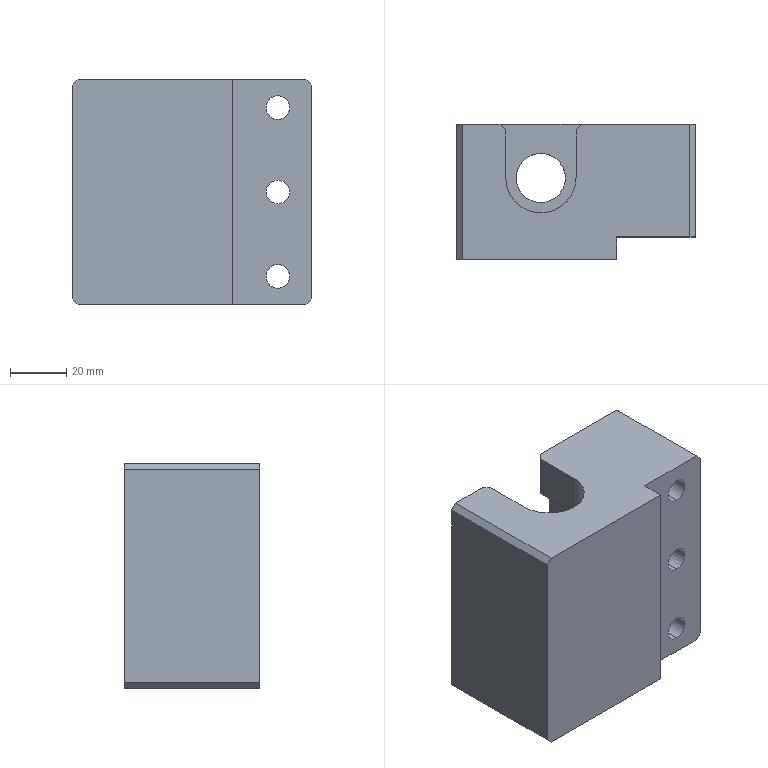Part | SolidWorks | features HoleWzd 2, ICE 2, Chamfer 1, Extrusion 1 | 1 solid | 39 faces | box 85 x 48 x 80 mm | volume 234146 mm3 | plane 23 | cylinder 16 | commonest cylinder face diameters 8.4 x6 15 x6 17.5 x2 25 x1 38 x1
STEP:
#1=CARTESIAN_POINT('',(36.037,-10.191,2.5));
#2=VERTEX_POINT('',#1);
#3=CARTESIAN_POINT('',(36.037,-10.191,17.5));
#4=VERTEX_POINT('',#3);
#5=CARTESIAN_POINT('',(36.037,-10.191,10.));
#6=DIRECTION('',(0.,1.,0.));
#7=DIRECTION('',(0.,0.,1.));
#8=AXIS2_PLACEMENT_3D('',#5,#6,#7);
#9=CIRCLE('',#8,7.5);
#10=EDGE_CURVE('',#2,#4,#9,.T.);
#11=ORIENTED_EDGE('',*,*,#10,.F.);
#12=CARTESIAN_POINT('',(36.037,9.809,2.5));
#13=VERTEX_POINT('',#12);
#14=CARTESIAN_POINT('',(36.037,9.809,2.5));
#15=DIRECTION('',(0.,1.,0.));
#16=VECTOR('',#15,1000.);
#17=LINE('',#14,#16);
#18=EDGE_CURVE('',#2,#13,#17,.T.);
#19=ORIENTED_EDGE('',*,*,#18,.T.);
#20=CARTESIAN_POINT('',(36.037,9.809,17.5));
#21=VERTEX_POINT('',#20);
#22=CARTESIAN_POINT('',(36.037,9.809,10.));
#23=DIRECTION('',(0.,1.,0.));
#24=DIRECTION('',(0.,0.,1.));
#25=AXIS2_PLACEMENT_3D('',#22,#23,#24);
#26=CIRCLE('',#25,7.5);
#27=EDGE_CURVE('',#13,#21,#26,.T.);
#28=ORIENTED_EDGE('',*,*,#27,.T.);
#29=CARTESIAN_POINT('',(36.037,9.809,17.5));
#30=DIRECTION('',(0.,1.,0.));
#31=VECTOR('',#30,1000.);
#32=LINE('',#29,#31);
#33=EDGE_CURVE('',#4,#21,#32,.T.);
#34=ORIENTED_EDGE('',*,*,#33,.F.);
#35=EDGE_LOOP('',(#11,#19,#28,#34));
#36=FACE_OUTER_BOUND('',#35,.T.);
#37=CARTESIAN_POINT('',(36.037,9.809,10.));
#38=DIRECTION('',(0.,1.,0.));
#39=DIRECTION('',(0.,0.,1.));
#40=AXIS2_PLACEMENT_3D('',#37,#38,#39);
#41=CYLINDRICAL_SURFACE('',#40,7.5);
#42=ADVANCED_FACE('',(#36),#41,.F.);
#43=CARTESIAN_POINT('',(36.037,-30.191,5.8));
#44=VERTEX_POINT('',#43);
#45=CARTESIAN_POINT('',(36.037,-30.191,14.2));
#46=VERTEX_POINT('',#45);
#47=CARTESIAN_POINT('',(36.037,-30.191,10.));
#48=DIRECTION('',(0.,1.,0.));
#49=DIRECTION('',(0.,0.,1.));
#50=AXIS2_PLACEMENT_3D('',#47,#48,#49);
#51=CIRCLE('',#50,4.2);
#52=EDGE_CURVE('',#44,#46,#51,.T.);
#53=ORIENTED_EDGE('',*,*,#52,.F.);
#54=CARTESIAN_POINT('',(36.037,-10.191,5.8));
#55=VERTEX_POINT('',#54);
#56=CARTESIAN_POINT('',(36.037,9.809,5.8));
#57=DIRECTION('',(0.,1.,0.));
#58=VECTOR('',#57,1000.);
#59=LINE('',#56,#58);
#60=EDGE_CURVE('',#44,#55,#59,.T.);
#61=ORIENTED_EDGE('',*,*,#60,.T.);
#62=CARTESIAN_POINT('',(36.037,-10.191,14.2));
#63=VERTEX_POINT('',#62);
#64=CARTESIAN_POINT('',(36.037,-10.191,10.));
#65=DIRECTION('',(0.,1.,0.));
#66=DIRECTION('',(0.,0.,1.));
#67=AXIS2_PLACEMENT_3D('',#64,#65,#66);
#68=CIRCLE('',#67,4.2);
#69=EDGE_CURVE('',#55,#63,#68,.T.);
#70=ORIENTED_EDGE('',*,*,#69,.T.);
#71=CARTESIAN_POINT('',(36.037,9.809,14.2));
#72=DIRECTION('',(0.,1.,0.));
#73=VECTOR('',#72,1000.);
#74=LINE('',#71,#73);
#75=EDGE_CURVE('',#46,#63,#74,.T.);
#76=ORIENTED_EDGE('',*,*,#75,.F.);
#77=EDGE_LOOP('',(#53,#61,#70,#76));
#78=FACE_OUTER_BOUND('',#77,.T.);
#79=CARTESIAN_POINT('',(36.037,9.809,10.));
#80=DIRECTION('',(0.,1.,0.));
#81=DIRECTION('',(0.,0.,1.));
#82=AXIS2_PLACEMENT_3D('',#79,#80,#81);
#83=CYLINDRICAL_SURFACE('',#82,4.2);
#84=ADVANCED_FACE('',(#78),#83,.F.);
#85=CARTESIAN_POINT('',(36.037,-10.191,32.5));
#86=VERTEX_POINT('',#85);
#87=CARTESIAN_POINT('',(36.037,-10.191,47.5));
#88=VERTEX_POINT('',#87);
#89=CARTESIAN_POINT('',(36.037,-10.191,40.));
#90=DIRECTION('',(0.,1.,0.));
#91=DIRECTION('',(0.,0.,1.));
#92=AXIS2_PLACEMENT_3D('',#89,#90,#91);
#93=CIRCLE('',#92,7.5);
#94=EDGE_CURVE('',#86,#88,#93,.T.);
#95=ORIENTED_EDGE('',*,*,#94,.F.);
#96=CARTESIAN_POINT('',(36.037,9.809,32.5));
#97=VERTEX_POINT('',#96);
#98=CARTESIAN_POINT('',(36.037,9.809,32.5));
#99=DIRECTION('',(0.,1.,0.));
#100=VECTOR('',#99,1000.);
#101=LINE('',#98,#100);
#102=EDGE_CURVE('',#86,#97,#101,.T.);
#103=ORIENTED_EDGE('',*,*,#102,.T.);
#104=CARTESIAN_POINT('',(36.037,9.809,47.5));
#105=VERTEX_POINT('',#104);
#106=CARTESIAN_POINT('',(36.037,9.809,40.));
#107=DIRECTION('',(0.,1.,0.));
#108=DIRECTION('',(0.,0.,1.));
#109=AXIS2_PLACEMENT_3D('',#106,#107,#108);
#110=CIRCLE('',#109,7.5);
#111=EDGE_CURVE('',#97,#105,#110,.T.);
#112=ORIENTED_EDGE('',*,*,#111,.T.);
#113=CARTESIAN_POINT('',(36.037,9.809,47.5));
#114=DIRECTION('',(0.,1.,0.));
#115=VECTOR('',#114,1000.);
#116=LINE('',#113,#115);
#117=EDGE_CURVE('',#88,#105,#116,.T.);
#118=ORIENTED_EDGE('',*,*,#117,.F.);
#119=EDGE_LOOP('',(#95,#103,#112,#118));
#120=FACE_OUTER_BOUND('',#119,.T.);
#121=CARTESIAN_POINT('',(36.037,9.809,40.));
#122=DIRECTION('',(0.,1.,0.));
#123=DIRECTION('',(0.,0.,1.));
#124=AXIS2_PLACEMENT_3D('',#121,#122,#123);
#125=CYLINDRICAL_SURFACE('',#124,7.5);
#126=ADVANCED_FACE('',(#120),#125,.F.);
#127=CARTESIAN_POINT('',(36.037,-30.191,35.8));
#128=VERTEX_POINT('',#127);
#129=CARTESIAN_POINT('',(36.037,-30.191,44.2));
#130=VERTEX_POINT('',#129);
#131=CARTESIAN_POINT('',(36.037,-30.191,40.));
#132=DIRECTION('',(0.,1.,0.));
#133=DIRECTION('',(0.,0.,1.));
#134=AXIS2_PLACEMENT_3D('',#131,#132,#133);
#135=CIRCLE('',#134,4.2);
#136=EDGE_CURVE('',#128,#130,#135,.T.);
#137=ORIENTED_EDGE('',*,*,#136,.F.);
#138=CARTESIAN_POINT('',(36.037,-10.191,35.8));
#139=VERTEX_POINT('',#138);
#140=CARTESIAN_POINT('',(36.037,9.809,35.8));
#141=DIRECTION('',(0.,1.,0.));
#142=VECTOR('',#141,1000.);
#143=LINE('',#140,#142);
#144=EDGE_CURVE('',#128,#139,#143,.T.);
#145=ORIENTED_EDGE('',*,*,#144,.T.);
#146=CARTESIAN_POINT('',(36.037,-10.191,44.2));
#147=VERTEX_POINT('',#146);
#148=CARTESIAN_POINT('',(36.037,-10.191,40.));
#149=DIRECTION('',(0.,1.,0.));
#150=DIRECTION('',(0.,0.,1.));
#151=AXIS2_PLACEMENT_3D('',#148,#149,#150);
#152=CIRCLE('',#151,4.2);
#153=EDGE_CURVE('',#139,#147,#152,.T.);
#154=ORIENTED_EDGE('',*,*,#153,.T.);
#155=CARTESIAN_POINT('',(36.037,9.809,44.2));
#156=DIRECTION('',(0.,1.,0.));
#157=VECTOR('',#156,1000.);
#158=LINE('',#155,#157);
#159=EDGE_CURVE('',#130,#147,#158,.T.);
#160=ORIENTED_EDGE('',*,*,#159,.F.);
#161=EDGE_LOOP('',(#137,#145,#154,#160));
#162=FACE_OUTER_BOUND('',#161,.T.);
#163=CARTESIAN_POINT('',(36.037,9.809,40.));
#164=DIRECTION('',(0.,1.,0.));
#165=DIRECTION('',(0.,0.,1.));
#166=AXIS2_PLACEMENT_3D('',#163,#164,#165);
#167=CYLINDRICAL_SURFACE('',#166,4.2);
#168=ADVANCED_FACE('',(#162),#167,.F.);
#169=CARTESIAN_POINT('',(36.037,-10.191,62.5));
#170=VERTEX_POINT('',#169);
#171=CARTESIAN_POINT('',(36.037,-10.191,77.5));
#172=VERTEX_POINT('',#171);
#173=CARTESIAN_POINT('',(36.037,-10.191,70.));
#174=DIRECTION('',(0.,1.,0.));
#175=DIRECTION('',(0.,0.,1.));
#176=AXIS2_PLACEMENT_3D('',#173,#174,#175);
#177=CIRCLE('',#176,7.5);
#178=EDGE_CURVE('',#170,#172,#177,.T.);
#179=ORIENTED_EDGE('',*,*,#178,.F.);
#180=CARTESIAN_POINT('',(36.037,9.809,62.5));
#181=VERTEX_POINT('',#180);
#182=CARTESIAN_POINT('',(36.037,9.809,62.5));
#183=DIRECTION('',(0.,1.,0.));
#184=VECTOR('',#183,1000.);
#185=LINE('',#182,#184);
#186=EDGE_CURVE('',#170,#181,#185,.T.);
#187=ORIENTED_EDGE('',*,*,#186,.T.);
#188=CARTESIAN_POINT('',(36.037,9.809,77.5));
#189=VERTEX_POINT('',#188);
#190=CARTESIAN_POINT('',(36.037,9.809,70.));
#191=DIRECTION('',(0.,1.,0.));
#192=DIRECTION('',(0.,0.,1.));
#193=AXIS2_PLACEMENT_3D('',#190,#191,#192);
#194=CIRCLE('',#193,7.5);
#195=EDGE_CURVE('',#181,#189,#194,.T.);
#196=ORIENTED_EDGE('',*,*,#195,.T.);
#197=CARTESIAN_POINT('',(36.037,9.809,77.5));
#198=DIRECTION('',(0.,1.,0.));
#199=VECTOR('',#198,1000.);
#200=LINE('',#197,#199);
#201=EDGE_CURVE('',#172,#189,#200,.T.);
#202=ORIENTED_EDGE('',*,*,#201,.F.);
#203=EDGE_LOOP('',(#179,#187,#196,#202));
#204=FACE_OUTER_BOUND('',#203,.T.);
#205=CARTESIAN_POINT('',(36.037,9.809,70.));
#206=DIRECTION('',(0.,1.,0.));
#207=DIRECTION('',(0.,0.,1.));
#208=AXIS2_PLACEMENT_3D('',#205,#206,#207);
#209=CYLINDRICAL_SURFACE('',#208,7.5);
#210=ADVANCED_FACE('',(#204),#209,.F.);
#211=CARTESIAN_POINT('',(36.037,-30.191,65.8));
#212=VERTEX_POINT('',#211);
#213=CARTESIAN_POINT('',(36.037,-30.191,74.2));
#214=VERTEX_POINT('',#213);
#215=CARTESIAN_POINT('',(36.037,-30.191,70.));
#216=DIRECTION('',(0.,1.,0.));
#217=DIRECTION('',(0.,0.,1.));
#218=AXIS2_PLACEMENT_3D('',#215,#216,#217);
#219=CIRCLE('',#218,4.2);
#220=EDGE_CURVE('',#212,#214,#219,.T.);
#221=ORIENTED_EDGE('',*,*,#220,.F.);
#222=CARTESIAN_POINT('',(36.037,-10.191,65.8));
#223=VERTEX_POINT('',#222);
#224=CARTESIAN_POINT('',(36.037,9.809,65.8));
#225=DIRECTION('',(0.,1.,0.));
#226=VECTOR('',#225,1000.);
#227=LINE('',#224,#226);
#228=EDGE_CURVE('',#212,#223,#227,.T.);
#229=ORIENTED_EDGE('',*,*,#228,.T.);
#230=CARTESIAN_POINT('',(36.037,-10.191,74.2));
#231=VERTEX_POINT('',#230);
#232=CARTESIAN_POINT('',(36.037,-10.191,70.));
#233=DIRECTION('',(0.,1.,0.));
#234=DIRECTION('',(0.,0.,1.));
#235=AXIS2_PLACEMENT_3D('',#232,#233,#234);
#236=CIRCLE('',#235,4.2);
#237=EDGE_CURVE('',#223,#231,#236,.T.);
#238=ORIENTED_EDGE('',*,*,#237,.T.);
#239=CARTESIAN_POINT('',(36.037,9.809,74.2));
#240=DIRECTION('',(0.,1.,0.));
#241=VECTOR('',#240,1000.);
#242=LINE('',#239,#241);
#243=EDGE_CURVE('',#214,#231,#242,.T.);
#244=ORIENTED_EDGE('',*,*,#243,.F.);
#245=EDGE_LOOP('',(#221,#229,#238,#244));
#246=FACE_OUTER_BOUND('',#245,.T.);
#247=CARTESIAN_POINT('',(36.037,9.809,70.));
#248=DIRECTION('',(0.,1.,0.));
#249=DIRECTION('',(0.,0.,1.));
#250=AXIS2_PLACEMENT_3D('',#247,#248,#249);
#251=CYLINDRICAL_SURFACE('',#250,4.2);
#252=ADVANCED_FACE('',(#246),#251,.F.);
#253=CARTESIAN_POINT('',(-15.713,-9.191,0.));
#254=VERTEX_POINT('',#253);
#255=CARTESIAN_POINT('',(1.787,-9.191,0.));
#256=VERTEX_POINT('',#255);
#257=CARTESIAN_POINT('',(-6.963,-9.191,0.));
#258=DIRECTION('',(0.,0.,1.));
#259=DIRECTION('',(1.,0.,0.));
#260=AXIS2_PLACEMENT_3D('',#257,#258,#259);
#261=CIRCLE('',#260,8.75);
#262=EDGE_CURVE('',#254,#256,#261,.T.);
#263=ORIENTED_EDGE('',*,*,#262,.F.);
#264=CARTESIAN_POINT('',(-15.713,-9.191,33.));
#265=VERTEX_POINT('',#264);
#266=CARTESIAN_POINT('',(-15.713,-9.191,33.));
#267=DIRECTION('',(0.,0.,1.));
#268=VECTOR('',#267,1000.);
#269=LINE('',#266,#268);
#270=EDGE_CURVE('',#254,#265,#269,.T.);
#271=ORIENTED_EDGE('',*,*,#270,.T.);
#272=CARTESIAN_POINT('',(1.787,-9.191,33.));
#273=VERTEX_POINT('',#272);
#274=CARTESIAN_POINT('',(-6.963,-9.191,33.));
#275=DIRECTION('',(0.,0.,1.));
#276=DIRECTION('',(1.,0.,0.));
#277=AXIS2_PLACEMENT_3D('',#274,#275,#276);
#278=CIRCLE('',#277,8.75);
#279=EDGE_CURVE('',#265,#273,#278,.T.);
#280=ORIENTED_EDGE('',*,*,#279,.T.);
#281=CARTESIAN_POINT('',(1.787,-9.191,33.));
#282=DIRECTION('',(0.,0.,1.));
#283=VECTOR('',#282,1000.);
#284=LINE('',#281,#283);
#285=EDGE_CURVE('',#256,#273,#284,.T.);
#286=ORIENTED_EDGE('',*,*,#285,.F.);
#287=EDGE_LOOP('',(#263,#271,#280,#286));
#288=FACE_OUTER_BOUND('',#287,.T.);
#289=CARTESIAN_POINT('',(-6.963,-9.191,33.));
#290=DIRECTION('',(0.,0.,1.));
#291=DIRECTION('',(1.,0.,0.));
#292=AXIS2_PLACEMENT_3D('',#289,#290,#291);
#293=CYLINDRICAL_SURFACE('',#292,8.75);
#294=ADVANCED_FACE('',(#288),#293,.F.);
#295=CARTESIAN_POINT('',(36.037,9.809,10.));
#296=DIRECTION('',(0.,1.,0.));
#297=DIRECTION('',(0.,0.,1.));
#298=AXIS2_PLACEMENT_3D('',#295,#296,#297);
#299=CIRCLE('',#298,7.5);
#300=EDGE_CURVE('',#21,#13,#299,.T.);
#301=ORIENTED_EDGE('',*,*,#300,.F.);
#302=ORIENTED_EDGE('',*,*,#27,.F.);
#303=EDGE_LOOP('',(#301,#302));
#304=FACE_BOUND('',#303,.T.);
#305=CARTESIAN_POINT('',(36.037,9.809,40.));
#306=DIRECTION('',(0.,1.,0.));
#307=DIRECTION('',(0.,0.,1.));
#308=AXIS2_PLACEMENT_3D('',#305,#306,#307);
#309=CIRCLE('',#308,7.5);
#310=EDGE_CURVE('',#105,#97,#309,.T.);
#311=ORIENTED_EDGE('',*,*,#310,.F.);
#312=ORIENTED_EDGE('',*,*,#111,.F.);
#313=EDGE_LOOP('',(#311,#312));
#314=FACE_BOUND('',#313,.T.);
#315=CARTESIAN_POINT('',(36.037,9.809,70.));
#316=DIRECTION('',(0.,1.,0.));
#317=DIRECTION('',(0.,0.,1.));
#318=AXIS2_PLACEMENT_3D('',#315,#316,#317);
#319=CIRCLE('',#318,7.5);
#320=EDGE_CURVE('',#189,#181,#319,.T.);
#321=ORIENTED_EDGE('',*,*,#320,.F.);
#322=ORIENTED_EDGE('',*,*,#195,.F.);
#323=EDGE_LOOP('',(#321,#322));
#324=FACE_BOUND('',#323,.T.);
#325=CARTESIAN_POINT('',(48.037,9.809,78.));
#326=VERTEX_POINT('',#325);
#327=CARTESIAN_POINT('',(48.037,9.809,2.));
#328=VERTEX_POINT('',#327);
#329=CARTESIAN_POINT('',(48.037,9.809,80.));
#330=DIRECTION('',(0.,0.,-1.));
#331=VECTOR('',#330,1000.);
#332=LINE('',#329,#331);
#333=EDGE_CURVE('',#326,#328,#332,.T.);
#334=ORIENTED_EDGE('',*,*,#333,.T.);
#335=CARTESIAN_POINT('',(46.037,9.809,0.));
#336=VERTEX_POINT('',#335);
#337=CARTESIAN_POINT('',(48.037,9.809,2.));
#338=DIRECTION('',(-0.7071,0.,-0.7071));
#339=VECTOR('',#338,1000.);
#340=LINE('',#337,#339);
#341=EDGE_CURVE('',#328,#336,#340,.T.);
#342=ORIENTED_EDGE('',*,*,#341,.T.);
#343=CARTESIAN_POINT('',(-34.963,9.809,0.));
#344=VERTEX_POINT('',#343);
#345=CARTESIAN_POINT('',(48.037,9.809,0.));
#346=DIRECTION('',(-1.,0.,0.));
#347=VECTOR('',#346,1000.);
#348=LINE('',#345,#347);
#349=EDGE_CURVE('',#336,#344,#348,.T.);
#350=ORIENTED_EDGE('',*,*,#349,.T.);
#351=CARTESIAN_POINT('',(-36.963,9.809,2.));
#352=VERTEX_POINT('',#351);
#353=CARTESIAN_POINT('',(-36.963,9.809,2.));
#354=DIRECTION('',(-0.7071,0.,0.7071));
#355=VECTOR('',#354,1000.);
#356=LINE('',#353,#355);
#357=EDGE_CURVE('',#344,#352,#356,.T.);
#358=ORIENTED_EDGE('',*,*,#357,.T.);
#359=CARTESIAN_POINT('',(-36.963,9.809,78.));
#360=VERTEX_POINT('',#359);
#361=CARTESIAN_POINT('',(-36.963,9.809,80.));
#362=DIRECTION('',(0.,0.,-1.));
#363=VECTOR('',#362,1000.);
#364=LINE('',#361,#363);
#365=EDGE_CURVE('',#360,#352,#364,.T.);
#366=ORIENTED_EDGE('',*,*,#365,.F.);
#367=CARTESIAN_POINT('',(-34.963,9.809,80.));
#368=VERTEX_POINT('',#367);
#369=CARTESIAN_POINT('',(-34.963,9.809,80.));
#370=DIRECTION('',(0.7071,0.,0.7071));
#371=VECTOR('',#370,1000.);
#372=LINE('',#369,#371);
#373=EDGE_CURVE('',#360,#368,#372,.T.);
#374=ORIENTED_EDGE('',*,*,#373,.T.);
#375=CARTESIAN_POINT('',(-21.463,9.809,80.));
#376=VERTEX_POINT('',#375);
#377=CARTESIAN_POINT('',(48.037,9.809,80.));
#378=DIRECTION('',(-1.,0.,0.));
#379=VECTOR('',#378,1000.);
#380=LINE('',#377,#379);
#381=EDGE_CURVE('',#376,#368,#380,.T.);
#382=ORIENTED_EDGE('',*,*,#381,.F.);
#383=CARTESIAN_POINT('',(-21.463,9.809,65.));
#384=VERTEX_POINT('',#383);
#385=CARTESIAN_POINT('',(-21.463,9.809,80.));
#386=DIRECTION('',(0.,0.,-1.));
#387=VECTOR('',#386,1000.);
#388=LINE('',#385,#387);
#389=EDGE_CURVE('',#376,#384,#388,.T.);
#390=ORIENTED_EDGE('',*,*,#389,.T.);
#391=CARTESIAN_POINT('',(-25.963,9.809,65.));
#392=VERTEX_POINT('',#391);
#393=CARTESIAN_POINT('',(-25.963,9.809,65.));
#394=DIRECTION('',(-1.,0.,0.));
#395=VECTOR('',#394,1000.);
#396=LINE('',#393,#395);
#397=EDGE_CURVE('',#384,#392,#396,.T.);
#398=ORIENTED_EDGE('',*,*,#397,.T.);
#399=CARTESIAN_POINT('',(-25.963,9.809,33.));
#400=VERTEX_POINT('',#399);
#401=CARTESIAN_POINT('',(-25.963,9.809,33.));
#402=DIRECTION('',(0.,0.,1.));
#403=VECTOR('',#402,1000.);
#404=LINE('',#401,#403);
#405=EDGE_CURVE('',#400,#392,#404,.T.);
#406=ORIENTED_EDGE('',*,*,#405,.F.);
#407=CARTESIAN_POINT('',(12.037,9.809,33.));
#408=VERTEX_POINT('',#407);
#409=CARTESIAN_POINT('',(-25.963,9.809,33.));
#410=DIRECTION('',(-1.,0.,0.));
#411=VECTOR('',#410,1000.);
#412=LINE('',#409,#411);
#413=EDGE_CURVE('',#408,#400,#412,.T.);
#414=ORIENTED_EDGE('',*,*,#413,.F.);
#415=CARTESIAN_POINT('',(12.037,9.809,65.));
#416=VERTEX_POINT('',#415);
#417=CARTESIAN_POINT('',(12.037,9.809,33.));
#418=DIRECTION('',(0.,0.,1.));
#419=VECTOR('',#418,1000.);
#420=LINE('',#417,#419);
#421=EDGE_CURVE('',#408,#416,#420,.T.);
#422=ORIENTED_EDGE('',*,*,#421,.T.);
#423=CARTESIAN_POINT('',(7.537,9.809,65.));
#424=VERTEX_POINT('',#423);
#425=CARTESIAN_POINT('',(-25.963,9.809,65.));
#426=DIRECTION('',(-1.,0.,0.));
#427=VECTOR('',#426,1000.);
#428=LINE('',#425,#427);
#429=EDGE_CURVE('',#416,#424,#428,.T.);
#430=ORIENTED_EDGE('',*,*,#429,.T.);
#431=CARTESIAN_POINT('',(7.537,9.809,80.));
#432=VERTEX_POINT('',#431);
#433=CARTESIAN_POINT('',(7.537,9.809,80.));
#434=DIRECTION('',(0.,0.,1.));
#435=VECTOR('',#434,1000.);
#436=LINE('',#433,#435);
#437=EDGE_CURVE('',#424,#432,#436,.T.);
#438=ORIENTED_EDGE('',*,*,#437,.T.);
#439=CARTESIAN_POINT('',(46.037,9.809,80.));
#440=VERTEX_POINT('',#439);
#441=CARTESIAN_POINT('',(48.037,9.809,80.));
#442=DIRECTION('',(-1.,0.,0.));
#443=VECTOR('',#442,1000.);
#444=LINE('',#441,#443);
#445=EDGE_CURVE('',#440,#432,#444,.T.);
#446=ORIENTED_EDGE('',*,*,#445,.F.);
#447=CARTESIAN_POINT('',(46.037,9.809,80.));
#448=DIRECTION('',(0.7071,0.,-0.7071));
#449=VECTOR('',#448,1000.);
#450=LINE('',#447,#449);
#451=EDGE_CURVE('',#440,#326,#450,.T.);
#452=ORIENTED_EDGE('',*,*,#451,.T.);
#453=EDGE_LOOP('',(#334,#342,#350,#358,#366,#374,#382,#390,#398,#406,#414,#422,#430,#438,#446,#452));
#454=FACE_OUTER_BOUND('',#453,.T.);
#455=CARTESIAN_POINT('',(48.037,9.809,80.));
#456=DIRECTION('',(0.,-1.,0.));
#457=DIRECTION('',(1.,0.,0.));
#458=AXIS2_PLACEMENT_3D('',#455,#456,#457);
#459=PLANE('',#458);
#460=ADVANCED_FACE('',(#304,#314,#324,#454),#459,.F.);
#461=ORIENTED_EDGE('',*,*,#365,.T.);
#462=CARTESIAN_POINT('',(-36.963,-38.191,2.));
#463=VERTEX_POINT('',#462);
#464=CARTESIAN_POINT('',(-36.963,9.809,2.));
#465=DIRECTION('',(0.,-1.,0.));
#466=VECTOR('',#465,1000.);
#467=LINE('',#464,#466);
#468=EDGE_CURVE('',#352,#463,#467,.T.);
#469=ORIENTED_EDGE('',*,*,#468,.T.);
#470=CARTESIAN_POINT('',(-36.963,-38.191,78.));
#471=VERTEX_POINT('',#470);
#472=CARTESIAN_POINT('',(-36.963,-38.191,80.));
#473=DIRECTION('',(0.,0.,-1.));
#474=VECTOR('',#473,1000.);
#475=LINE('',#472,#474);
#476=EDGE_CURVE('',#471,#463,#475,.T.);
#477=ORIENTED_EDGE('',*,*,#476,.F.);
#478=CARTESIAN_POINT('',(-36.963,9.809,78.));
#479=DIRECTION('',(0.,1.,0.));
#480=VECTOR('',#479,1000.);
#481=LINE('',#478,#480);
#482=EDGE_CURVE('',#471,#360,#481,.T.);
#483=ORIENTED_EDGE('',*,*,#482,.T.);
#484=EDGE_LOOP('',(#461,#469,#477,#483));
#485=FACE_OUTER_BOUND('',#484,.T.);
#486=CARTESIAN_POINT('',(-36.963,9.809,80.));
#487=DIRECTION('',(1.,0.,0.));
#488=DIRECTION('',(0.,0.,-1.));
#489=AXIS2_PLACEMENT_3D('',#486,#487,#488);
#490=PLANE('',#489);
#491=ADVANCED_FACE('',(#485),#490,.F.);
#492=ORIENTED_EDGE('',*,*,#476,.T.);
#493=CARTESIAN_POINT('',(-34.963,-38.191,0.));
#494=VERTEX_POINT('',#493);
#495=CARTESIAN_POINT('',(-36.963,-38.191,2.));
#496=DIRECTION('',(0.7071,0.,-0.7071));
#497=VECTOR('',#496,1000.);
#498=LINE('',#495,#497);
#499=EDGE_CURVE('',#463,#494,#498,.T.);
#500=ORIENTED_EDGE('',*,*,#499,.T.);
#501=CARTESIAN_POINT('',(20.037,-38.191,0.));
#502=VERTEX_POINT('',#501);
#503=CARTESIAN_POINT('',(-36.963,-38.191,0.));
#504=DIRECTION('',(1.,0.,0.));
#505=VECTOR('',#504,1000.);
#506=LINE('',#503,#505);
#507=EDGE_CURVE('',#494,#502,#506,.T.);
#508=ORIENTED_EDGE('',*,*,#507,.T.);
#509=CARTESIAN_POINT('',(20.037,-38.191,80.));
#510=VERTEX_POINT('',#509);
#511=CARTESIAN_POINT('',(20.037,-38.191,80.));
#512=DIRECTION('',(0.,0.,-1.));
#513=VECTOR('',#512,1000.);
#514=LINE('',#511,#513);
#515=EDGE_CURVE('',#510,#502,#514,.T.);
#516=ORIENTED_EDGE('',*,*,#515,.F.);
#517=CARTESIAN_POINT('',(-34.963,-38.191,80.));
#518=VERTEX_POINT('',#517);
#519=CARTESIAN_POINT('',(-36.963,-38.191,80.));
#520=DIRECTION('',(1.,0.,0.));
#521=VECTOR('',#520,1000.);
#522=LINE('',#519,#521);
#523=EDGE_CURVE('',#518,#510,#522,.T.);
#524=ORIENTED_EDGE('',*,*,#523,.F.);
#525=CARTESIAN_POINT('',(-34.963,-38.191,80.));
#526=DIRECTION('',(-0.7071,0.,-0.7071));
#527=VECTOR('',#526,1000.);
#528=LINE('',#525,#527);
#529=EDGE_CURVE('',#518,#471,#528,.T.);
#530=ORIENTED_EDGE('',*,*,#529,.T.);
#531=EDGE_LOOP('',(#492,#500,#508,#516,#524,#530));
#532=FACE_OUTER_BOUND('',#531,.T.);
#533=CARTESIAN_POINT('',(-36.963,-38.191,80.));
#534=DIRECTION('',(0.,1.,0.));
#535=DIRECTION('',(0.,0.,1.));
#536=AXIS2_PLACEMENT_3D('',#533,#534,#535);
#537=PLANE('',#536);
#538=ADVANCED_FACE('',(#532),#537,.F.);
#539=CARTESIAN_POINT('',(20.037,-30.191,0.));
#540=VERTEX_POINT('',#539);
#541=CARTESIAN_POINT('',(20.037,-38.191,0.));
#542=DIRECTION('',(0.,1.,0.));
#543=VECTOR('',#542,1000.);
#544=LINE('',#541,#543);
#545=EDGE_CURVE('',#502,#540,#544,.T.);
#546=ORIENTED_EDGE('',*,*,#545,.T.);
#547=CARTESIAN_POINT('',(20.037,-30.191,80.));
#548=VERTEX_POINT('',#547);
#549=CARTESIAN_POINT('',(20.037,-30.191,80.));
#550=DIRECTION('',(0.,0.,-1.));
#551=VECTOR('',#550,1000.);
#552=LINE('',#549,#551);
#553=EDGE_CURVE('',#548,#540,#552,.T.);
#554=ORIENTED_EDGE('',*,*,#553,.F.);
#555=CARTESIAN_POINT('',(20.037,-38.191,80.));
#556=DIRECTION('',(0.,1.,0.));
#557=VECTOR('',#556,1000.);
#558=LINE('',#555,#557);
#559=EDGE_CURVE('',#510,#548,#558,.T.);
#560=ORIENTED_EDGE('',*,*,#559,.F.);
#561=ORIENTED_EDGE('',*,*,#515,.T.);
#562=EDGE_LOOP('',(#546,#554,#560,#561));
#563=FACE_OUTER_BOUND('',#562,.T.);
#564=CARTESIAN_POINT('',(20.037,-38.191,80.));
#565=DIRECTION('',(-1.,0.,0.));
#566=DIRECTION('',(0.,0.,1.));
#567=AXIS2_PLACEMENT_3D('',#564,#565,#566);
#568=PLANE('',#567);
#569=ADVANCED_FACE('',(#563),#568,.F.);
#570=CARTESIAN_POINT('',(36.037,-30.191,10.));
#571=DIRECTION('',(0.,1.,0.));
#572=DIRECTION('',(0.,0.,1.));
#573=AXIS2_PLACEMENT_3D('',#570,#571,#572);
#574=CIRCLE('',#573,4.2);
#575=EDGE_CURVE('',#46,#44,#574,.T.);
#576=ORIENTED_EDGE('',*,*,#575,.T.);
#577=ORIENTED_EDGE('',*,*,#52,.T.);
#578=EDGE_LOOP('',(#576,#577));
#579=FACE_BOUND('',#578,.T.);
#580=CARTESIAN_POINT('',(36.037,-30.191,40.));
#581=DIRECTION('',(0.,1.,0.));
#582=DIRECTION('',(0.,0.,1.));
#583=AXIS2_PLACEMENT_3D('',#580,#581,#582);
#584=CIRCLE('',#583,4.2);
#585=EDGE_CURVE('',#130,#128,#584,.T.);
#586=ORIENTED_EDGE('',*,*,#585,.T.);
#587=ORIENTED_EDGE('',*,*,#136,.T.);
#588=EDGE_LOOP('',(#586,#587));
#589=FACE_BOUND('',#588,.T.);
#590=CARTESIAN_POINT('',(36.037,-30.191,70.));
#591=DIRECTION('',(0.,1.,0.));
#592=DIRECTION('',(0.,0.,1.));
#593=AXIS2_PLACEMENT_3D('',#590,#591,#592);
#594=CIRCLE('',#593,4.2);
#595=EDGE_CURVE('',#214,#212,#594,.T.);
#596=ORIENTED_EDGE('',*,*,#595,.T.);
#597=ORIENTED_EDGE('',*,*,#220,.T.);
#598=EDGE_LOOP('',(#596,#597));
#599=FACE_BOUND('',#598,.T.);
#600=CARTESIAN_POINT('',(46.037,-30.191,0.));
#601=VERTEX_POINT('',#600);
#602=CARTESIAN_POINT('',(20.037,-30.191,0.));
#603=DIRECTION('',(1.,0.,0.));
#604=VECTOR('',#603,1000.);
#605=LINE('',#602,#604);
#606=EDGE_CURVE('',#540,#601,#605,.T.);
#607=ORIENTED_EDGE('',*,*,#606,.T.);
#608=CARTESIAN_POINT('',(48.037,-30.191,2.));
#609=VERTEX_POINT('',#608);
#610=CARTESIAN_POINT('',(48.037,-30.191,2.));
#611=DIRECTION('',(0.7071,0.,0.7071));
#612=VECTOR('',#611,1000.);
#613=LINE('',#610,#612);
#614=EDGE_CURVE('',#601,#609,#613,.T.);
#615=ORIENTED_EDGE('',*,*,#614,.T.);
#616=CARTESIAN_POINT('',(48.037,-30.191,78.));
#617=VERTEX_POINT('',#616);
#618=CARTESIAN_POINT('',(48.037,-30.191,80.));
#619=DIRECTION('',(0.,0.,-1.));
#620=VECTOR('',#619,1000.);
#621=LINE('',#618,#620);
#622=EDGE_CURVE('',#617,#609,#621,.T.);
#623=ORIENTED_EDGE('',*,*,#622,.F.);
#624=CARTESIAN_POINT('',(46.037,-30.191,80.));
#625=VERTEX_POINT('',#624);
#626=CARTESIAN_POINT('',(46.037,-30.191,80.));
#627=DIRECTION('',(-0.7071,0.,0.7071));
#628=VECTOR('',#627,1000.);
#629=LINE('',#626,#628);
#630=EDGE_CURVE('',#617,#625,#629,.T.);
#631=ORIENTED_EDGE('',*,*,#630,.T.);
#632=CARTESIAN_POINT('',(20.037,-30.191,80.));
#633=DIRECTION('',(1.,0.,0.));
#634=VECTOR('',#633,1000.);
#635=LINE('',#632,#634);
#636=EDGE_CURVE('',#548,#625,#635,.T.);
#637=ORIENTED_EDGE('',*,*,#636,.F.);
#638=ORIENTED_EDGE('',*,*,#553,.T.);
#639=EDGE_LOOP('',(#607,#615,#623,#631,#637,#638));
#640=FACE_OUTER_BOUND('',#639,.T.);
#641=CARTESIAN_POINT('',(20.037,-30.191,80.));
#642=DIRECTION('',(0.,1.,0.));
#643=DIRECTION('',(0.,0.,1.));
#644=AXIS2_PLACEMENT_3D('',#641,#642,#643);
#645=PLANE('',#644);
#646=ADVANCED_FACE('',(#579,#589,#599,#640),#645,.F.);
#647=ORIENTED_EDGE('',*,*,#622,.T.);
#648=CARTESIAN_POINT('',(48.037,-30.191,2.));
#649=DIRECTION('',(0.,1.,0.));
#650=VECTOR('',#649,1000.);
#651=LINE('',#648,#650);
#652=EDGE_CURVE('',#609,#328,#651,.T.);
#653=ORIENTED_EDGE('',*,*,#652,.T.);
#654=ORIENTED_EDGE('',*,*,#333,.F.);
#655=CARTESIAN_POINT('',(48.037,-30.191,78.));
#656=DIRECTION('',(0.,-1.,0.));
#657=VECTOR('',#656,1000.);
#658=LINE('',#655,#657);
#659=EDGE_CURVE('',#326,#617,#658,.T.);
#660=ORIENTED_EDGE('',*,*,#659,.T.);
#661=EDGE_LOOP('',(#647,#653,#654,#660));
#662=FACE_OUTER_BOUND('',#661,.T.);
#663=CARTESIAN_POINT('',(48.037,-30.191,80.));
#664=DIRECTION('',(-1.,0.,0.));
#665=DIRECTION('',(0.,-1.,0.));
#666=AXIS2_PLACEMENT_3D('',#663,#664,#665);
#667=PLANE('',#666);
#668=ADVANCED_FACE('',(#662),#667,.F.);
#669=ORIENTED_EDGE('',*,*,#636,.T.);
#670=CARTESIAN_POINT('',(46.037,9.809,80.));
#671=DIRECTION('',(0.,1.,0.));
#672=VECTOR('',#671,1000.);
#673=LINE('',#670,#672);
#674=EDGE_CURVE('',#625,#440,#673,.T.);
#675=ORIENTED_EDGE('',*,*,#674,.T.);
#676=ORIENTED_EDGE('',*,*,#445,.T.);
#677=CARTESIAN_POINT('',(5.537,7.809,80.));
#678=VERTEX_POINT('',#677);
#679=CARTESIAN_POINT('',(-1.136,1.136,80.));
#680=DIRECTION('',(-0.7071,-0.7071,0.));
#681=VECTOR('',#680,1000.);
#682=LINE('',#679,#681);
#683=EDGE_CURVE('',#432,#678,#682,.T.);
#684=ORIENTED_EDGE('',*,*,#683,.T.);
#685=CARTESIAN_POINT('',(5.537,-9.191,80.));
#686=VERTEX_POINT('',#685);
#687=CARTESIAN_POINT('',(5.537,-9.191,80.));
#688=DIRECTION('',(0.,1.,0.));
#689=VECTOR('',#688,1000.);
#690=LINE('',#687,#689);
#691=EDGE_CURVE('',#686,#678,#690,.T.);
#692=ORIENTED_EDGE('',*,*,#691,.F.);
#693=CARTESIAN_POINT('',(-19.463,-9.191,80.));
#694=VERTEX_POINT('',#693);
#695=CARTESIAN_POINT('',(-6.963,-9.191,80.));
#696=DIRECTION('',(0.,0.,1.));
#697=DIRECTION('',(1.,0.,0.));
#698=AXIS2_PLACEMENT_3D('',#695,#696,#697);
#699=CIRCLE('',#698,12.5);
#700=EDGE_CURVE('',#694,#686,#699,.T.);
#701=ORIENTED_EDGE('',*,*,#700,.F.);
#702=CARTESIAN_POINT('',(-19.463,7.809,80.));
#703=VERTEX_POINT('',#702);
#704=CARTESIAN_POINT('',(-19.463,-9.191,80.));
#705=DIRECTION('',(0.,-1.,0.));
#706=VECTOR('',#705,1000.);
#707=LINE('',#704,#706);
#708=EDGE_CURVE('',#703,#694,#707,.T.);
#709=ORIENTED_EDGE('',*,*,#708,.F.);
#710=CARTESIAN_POINT('',(-5.827,-5.827,80.));
#711=DIRECTION('',(-0.7071,0.7071,0.));
#712=VECTOR('',#711,1000.);
#713=LINE('',#710,#712);
#714=EDGE_CURVE('',#703,#376,#713,.T.);
#715=ORIENTED_EDGE('',*,*,#714,.T.);
#716=ORIENTED_EDGE('',*,*,#381,.T.);
#717=CARTESIAN_POINT('',(-34.963,-38.191,80.));
#718=DIRECTION('',(0.,-1.,0.));
#719=VECTOR('',#718,1000.);
#720=LINE('',#717,#719);
#721=EDGE_CURVE('',#368,#518,#720,.T.);
#722=ORIENTED_EDGE('',*,*,#721,.T.);
#723=ORIENTED_EDGE('',*,*,#523,.T.);
#724=ORIENTED_EDGE('',*,*,#559,.T.);
#725=EDGE_LOOP('',(#669,#675,#676,#684,#692,#701,#709,#715,#716,#722,#723,#724));
#726=FACE_OUTER_BOUND('',#725,.T.);
#727=CARTESIAN_POINT('',(0.,0.,80.));
#728=DIRECTION('',(0.,0.,1.));
#729=DIRECTION('',(1.,0.,0.));
#730=AXIS2_PLACEMENT_3D('',#727,#728,#729);
#731=PLANE('',#730);
#732=ADVANCED_FACE('',(#726),#731,.T.);
#733=CARTESIAN_POINT('',(-6.963,-9.191,0.));
#734=DIRECTION('',(0.,0.,1.));
#735=DIRECTION('',(1.,0.,0.));
#736=AXIS2_PLACEMENT_3D('',#733,#734,#735);
#737=CIRCLE('',#736,8.75);
#738=EDGE_CURVE('',#256,#254,#737,.T.);
#739=ORIENTED_EDGE('',*,*,#738,.T.);
#740=ORIENTED_EDGE('',*,*,#262,.T.);
#741=EDGE_LOOP('',(#739,#740));
#742=FACE_BOUND('',#741,.T.);
#743=ORIENTED_EDGE('',*,*,#349,.F.);
#744=CARTESIAN_POINT('',(46.037,0.,0.));
#745=DIRECTION('',(0.,-1.,0.));
#746=VECTOR('',#745,1000.);
#747=LINE('',#744,#746);
#748=EDGE_CURVE('',#336,#601,#747,.T.);
#749=ORIENTED_EDGE('',*,*,#748,.T.);
#750=ORIENTED_EDGE('',*,*,#606,.F.);
#751=ORIENTED_EDGE('',*,*,#545,.F.);
#752=ORIENTED_EDGE('',*,*,#507,.F.);
#753=CARTESIAN_POINT('',(-34.963,0.,0.));
#754=DIRECTION('',(0.,1.,0.));
#755=VECTOR('',#754,1000.);
#756=LINE('',#753,#755);
#757=EDGE_CURVE('',#494,#344,#756,.T.);
#758=ORIENTED_EDGE('',*,*,#757,.T.);
#759=EDGE_LOOP('',(#743,#749,#750,#751,#752,#758));
#760=FACE_OUTER_BOUND('',#759,.T.);
#761=CARTESIAN_POINT('',(0.,0.,0.));
#762=DIRECTION('',(0.,0.,1.));
#763=DIRECTION('',(1.,0.,0.));
#764=AXIS2_PLACEMENT_3D('',#761,#762,#763);
#765=PLANE('',#764);
#766=ADVANCED_FACE('',(#742,#760),#765,.F.);
#767=ORIENTED_EDGE('',*,*,#700,.T.);
#768=CARTESIAN_POINT('',(5.537,-9.191,65.));
#769=VERTEX_POINT('',#768);
#770=CARTESIAN_POINT('',(5.537,-9.191,65.));
#771=DIRECTION('',(0.,0.,1.));
#772=VECTOR('',#771,1000.);
#773=LINE('',#770,#772);
#774=EDGE_CURVE('',#769,#686,#773,.T.);
#775=ORIENTED_EDGE('',*,*,#774,.F.);
#776=CARTESIAN_POINT('',(-19.463,-9.191,65.));
#777=VERTEX_POINT('',#776);
#778=CARTESIAN_POINT('',(-6.963,-9.191,65.));
#779=DIRECTION('',(0.,0.,1.));
#780=DIRECTION('',(1.,0.,0.));
#781=AXIS2_PLACEMENT_3D('',#778,#779,#780);
#782=CIRCLE('',#781,12.5);
#783=EDGE_CURVE('',#777,#769,#782,.T.);
#784=ORIENTED_EDGE('',*,*,#783,.F.);
#785=CARTESIAN_POINT('',(-19.463,-9.191,65.));
#786=DIRECTION('',(0.,0.,1.));
#787=VECTOR('',#786,1000.);
#788=LINE('',#785,#787);
#789=EDGE_CURVE('',#777,#694,#788,.T.);
#790=ORIENTED_EDGE('',*,*,#789,.T.);
#791=EDGE_LOOP('',(#767,#775,#784,#790));
#792=FACE_OUTER_BOUND('',#791,.T.);
#793=CARTESIAN_POINT('',(-6.963,-9.191,65.));
#794=DIRECTION('',(0.,0.,1.));
#795=DIRECTION('',(1.,0.,0.));
#796=AXIS2_PLACEMENT_3D('',#793,#794,#795);
#797=CYLINDRICAL_SURFACE('',#796,12.5);
#798=ADVANCED_FACE('',(#792),#797,.F.);
#799=CARTESIAN_POINT('',(-19.463,7.809,65.));
#800=VERTEX_POINT('',#799);
#801=CARTESIAN_POINT('',(-19.463,-9.191,65.));
#802=DIRECTION('',(0.,-1.,0.));
#803=VECTOR('',#802,1000.);
#804=LINE('',#801,#803);
#805=EDGE_CURVE('',#800,#777,#804,.T.);
#806=ORIENTED_EDGE('',*,*,#805,.F.);
#807=CARTESIAN_POINT('',(-19.463,7.809,65.));
#808=DIRECTION('',(0.,0.,1.));
#809=VECTOR('',#808,1000.);
#810=LINE('',#807,#809);
#811=EDGE_CURVE('',#800,#703,#810,.T.);
#812=ORIENTED_EDGE('',*,*,#811,.T.);
#813=ORIENTED_EDGE('',*,*,#708,.T.);
#814=ORIENTED_EDGE('',*,*,#789,.F.);
#815=EDGE_LOOP('',(#806,#812,#813,#814));
#816=FACE_OUTER_BOUND('',#815,.T.);
#817=CARTESIAN_POINT('',(-19.463,-9.191,65.));
#818=DIRECTION('',(-1.,0.,0.));
#819=DIRECTION('',(0.,-1.,0.));
#820=AXIS2_PLACEMENT_3D('',#817,#818,#819);
#821=PLANE('',#820);
#822=ADVANCED_FACE('',(#816),#821,.F.);
#823=ORIENTED_EDGE('',*,*,#691,.T.);
#824=CARTESIAN_POINT('',(5.537,7.809,65.));
#825=VERTEX_POINT('',#824);
#826=CARTESIAN_POINT('',(5.537,7.809,65.));
#827=DIRECTION('',(0.,0.,-1.));
#828=VECTOR('',#827,1000.);
#829=LINE('',#826,#828);
#830=EDGE_CURVE('',#678,#825,#829,.T.);
#831=ORIENTED_EDGE('',*,*,#830,.T.);
#832=CARTESIAN_POINT('',(5.537,-9.191,65.));
#833=DIRECTION('',(0.,1.,0.));
#834=VECTOR('',#833,1000.);
#835=LINE('',#832,#834);
#836=EDGE_CURVE('',#769,#825,#835,.T.);
#837=ORIENTED_EDGE('',*,*,#836,.F.);
#838=ORIENTED_EDGE('',*,*,#774,.T.);
#839=EDGE_LOOP('',(#823,#831,#837,#838));
#840=FACE_OUTER_BOUND('',#839,.T.);
#841=CARTESIAN_POINT('',(5.537,-9.191,65.));
#842=DIRECTION('',(1.,0.,0.));
#843=DIRECTION('',(0.,1.,0.));
#844=AXIS2_PLACEMENT_3D('',#841,#842,#843);
#845=PLANE('',#844);
#846=ADVANCED_FACE('',(#840),#845,.F.);
#847=ORIENTED_EDGE('',*,*,#836,.T.);
#848=CARTESIAN_POINT('',(7.537,9.809,65.));
#849=DIRECTION('',(0.7071,0.7071,0.));
#850=VECTOR('',#849,1000.);
#851=LINE('',#848,#850);
#852=EDGE_CURVE('',#825,#424,#851,.T.);
#853=ORIENTED_EDGE('',*,*,#852,.T.);
#854=ORIENTED_EDGE('',*,*,#429,.F.);
#855=CARTESIAN_POINT('',(12.037,-9.191,65.));
#856=VERTEX_POINT('',#855);
#857=CARTESIAN_POINT('',(12.037,9.809,65.));
#858=DIRECTION('',(0.,1.,0.));
#859=VECTOR('',#858,1000.);
#860=LINE('',#857,#859);
#861=EDGE_CURVE('',#856,#416,#860,.T.);
#862=ORIENTED_EDGE('',*,*,#861,.F.);
#863=CARTESIAN_POINT('',(-25.963,-9.191,65.));
#864=VERTEX_POINT('',#863);
#865=CARTESIAN_POINT('',(-6.963,-9.191,65.));
#866=DIRECTION('',(0.,0.,1.));
#867=DIRECTION('',(1.,0.,0.));
#868=AXIS2_PLACEMENT_3D('',#865,#866,#867);
#869=CIRCLE('',#868,19.);
#870=EDGE_CURVE('',#864,#856,#869,.T.);
#871=ORIENTED_EDGE('',*,*,#870,.F.);
#872=CARTESIAN_POINT('',(-25.963,-9.191,65.));
#873=DIRECTION('',(0.,-1.,0.));
#874=VECTOR('',#873,1000.);
#875=LINE('',#872,#874);
#876=EDGE_CURVE('',#392,#864,#875,.T.);
#877=ORIENTED_EDGE('',*,*,#876,.F.);
#878=ORIENTED_EDGE('',*,*,#397,.F.);
#879=CARTESIAN_POINT('',(-19.463,7.809,65.));
#880=DIRECTION('',(0.7071,-0.7071,0.));
#881=VECTOR('',#880,1000.);
#882=LINE('',#879,#881);
#883=EDGE_CURVE('',#384,#800,#882,.T.);
#884=ORIENTED_EDGE('',*,*,#883,.T.);
#885=ORIENTED_EDGE('',*,*,#805,.T.);
#886=ORIENTED_EDGE('',*,*,#783,.T.);
#887=EDGE_LOOP('',(#847,#853,#854,#862,#871,#877,#878,#884,#885,#886));
#888=FACE_OUTER_BOUND('',#887,.T.);
#889=CARTESIAN_POINT('',(-6.963,-9.191,65.));
#890=DIRECTION('',(0.,0.,1.));
#891=DIRECTION('',(1.,0.,0.));
#892=AXIS2_PLACEMENT_3D('',#889,#890,#891);
#893=PLANE('',#892);
#894=ADVANCED_FACE('',(#888),#893,.F.);
#895=ORIENTED_EDGE('',*,*,#870,.T.);
#896=CARTESIAN_POINT('',(12.037,-9.191,33.));
#897=VERTEX_POINT('',#896);
#898=CARTESIAN_POINT('',(12.037,-9.191,33.));
#899=DIRECTION('',(0.,0.,1.));
#900=VECTOR('',#899,1000.);
#901=LINE('',#898,#900);
#902=EDGE_CURVE('',#897,#856,#901,.T.);
#903=ORIENTED_EDGE('',*,*,#902,.F.);
#904=CARTESIAN_POINT('',(-25.963,-9.191,33.));
#905=VERTEX_POINT('',#904);
#906=CARTESIAN_POINT('',(-6.963,-9.191,33.));
#907=DIRECTION('',(0.,0.,1.));
#908=DIRECTION('',(1.,0.,0.));
#909=AXIS2_PLACEMENT_3D('',#906,#907,#908);
#910=CIRCLE('',#909,19.);
#911=EDGE_CURVE('',#905,#897,#910,.T.);
#912=ORIENTED_EDGE('',*,*,#911,.F.);
#913=CARTESIAN_POINT('',(-25.963,-9.191,33.));
#914=DIRECTION('',(0.,0.,1.));
#915=VECTOR('',#914,1000.);
#916=LINE('',#913,#915);
#917=EDGE_CURVE('',#905,#864,#916,.T.);
#918=ORIENTED_EDGE('',*,*,#917,.T.);
#919=EDGE_LOOP('',(#895,#903,#912,#918));
#920=FACE_OUTER_BOUND('',#919,.T.);
#921=CARTESIAN_POINT('',(-6.963,-9.191,33.));
#922=DIRECTION('',(0.,0.,1.));
#923=DIRECTION('',(1.,0.,0.));
#924=AXIS2_PLACEMENT_3D('',#921,#922,#923);
#925=CYLINDRICAL_SURFACE('',#924,19.);
#926=ADVANCED_FACE('',(#920),#925,.F.);
#927=ORIENTED_EDGE('',*,*,#876,.T.);
#928=ORIENTED_EDGE('',*,*,#917,.F.);
#929=CARTESIAN_POINT('',(-25.963,-9.191,33.));
#930=DIRECTION('',(0.,-1.,0.));
#931=VECTOR('',#930,1000.);
#932=LINE('',#929,#931);
#933=EDGE_CURVE('',#400,#905,#932,.T.);
#934=ORIENTED_EDGE('',*,*,#933,.F.);
#935=ORIENTED_EDGE('',*,*,#405,.T.);
#936=EDGE_LOOP('',(#927,#928,#934,#935));
#937=FACE_OUTER_BOUND('',#936,.T.);
#938=CARTESIAN_POINT('',(-25.963,-9.191,33.));
#939=DIRECTION('',(-1.,0.,0.));
#940=DIRECTION('',(0.,0.,1.));
#941=AXIS2_PLACEMENT_3D('',#938,#939,#940);
#942=PLANE('',#941);
#943=ADVANCED_FACE('',(#937),#942,.F.);
#944=ORIENTED_EDGE('',*,*,#861,.T.);
#945=ORIENTED_EDGE('',*,*,#421,.F.);
#946=CARTESIAN_POINT('',(12.037,9.809,33.));
#947=DIRECTION('',(0.,1.,0.));
#948=VECTOR('',#947,1000.);
#949=LINE('',#946,#948);
#950=EDGE_CURVE('',#897,#408,#949,.T.);
#951=ORIENTED_EDGE('',*,*,#950,.F.);
#952=ORIENTED_EDGE('',*,*,#902,.T.);
#953=EDGE_LOOP('',(#944,#945,#951,#952));
#954=FACE_OUTER_BOUND('',#953,.T.);
#955=CARTESIAN_POINT('',(12.037,9.809,33.));
#956=DIRECTION('',(1.,0.,0.));
#957=DIRECTION('',(0.,1.,0.));
#958=AXIS2_PLACEMENT_3D('',#955,#956,#957);
#959=PLANE('',#958);
#960=ADVANCED_FACE('',(#954),#959,.F.);
#961=CARTESIAN_POINT('',(-6.963,-9.191,33.));
#962=DIRECTION('',(0.,0.,1.));
#963=DIRECTION('',(1.,0.,0.));
#964=AXIS2_PLACEMENT_3D('',#961,#962,#963);
#965=CIRCLE('',#964,8.75);
#966=EDGE_CURVE('',#273,#265,#965,.T.);
#967=ORIENTED_EDGE('',*,*,#966,.F.);
#968=ORIENTED_EDGE('',*,*,#279,.F.);
#969=EDGE_LOOP('',(#967,#968));
#970=FACE_BOUND('',#969,.T.);
#971=ORIENTED_EDGE('',*,*,#911,.T.);
#972=ORIENTED_EDGE('',*,*,#950,.T.);
#973=ORIENTED_EDGE('',*,*,#413,.T.);
#974=ORIENTED_EDGE('',*,*,#933,.T.);
#975=EDGE_LOOP('',(#971,#972,#973,#974));
#976=FACE_OUTER_BOUND('',#975,.T.);
#977=CARTESIAN_POINT('',(-6.963,-9.191,33.));
#978=DIRECTION('',(0.,0.,1.));
#979=DIRECTION('',(1.,0.,0.));
#980=AXIS2_PLACEMENT_3D('',#977,#978,#979);
#981=PLANE('',#980);
#982=ADVANCED_FACE('',(#970,#976),#981,.T.);
#983=ORIENTED_EDGE('',*,*,#270,.F.);
#984=ORIENTED_EDGE('',*,*,#738,.F.);
#985=ORIENTED_EDGE('',*,*,#285,.T.);
#986=ORIENTED_EDGE('',*,*,#966,.T.);
#987=EDGE_LOOP('',(#983,#984,#985,#986));
#988=FACE_OUTER_BOUND('',#987,.T.);
#989=CARTESIAN_POINT('',(-6.963,-9.191,33.));
#990=DIRECTION('',(0.,0.,1.));
#991=DIRECTION('',(1.,0.,0.));
#992=AXIS2_PLACEMENT_3D('',#989,#990,#991);
#993=CYLINDRICAL_SURFACE('',#992,8.75);
#994=ADVANCED_FACE('',(#988),#993,.F.);
#995=ORIENTED_EDGE('',*,*,#228,.F.);
#996=ORIENTED_EDGE('',*,*,#595,.F.);
#997=ORIENTED_EDGE('',*,*,#243,.T.);
#998=CARTESIAN_POINT('',(36.037,-10.191,70.));
#999=DIRECTION('',(0.,1.,0.));
#1000=DIRECTION('',(0.,0.,1.));
#1001=AXIS2_PLACEMENT_3D('',#998,#999,#1000);
#1002=CIRCLE('',#1001,4.2);
#1003=EDGE_CURVE('',#231,#223,#1002,.T.);
#1004=ORIENTED_EDGE('',*,*,#1003,.T.);
#1005=EDGE_LOOP('',(#995,#996,#997,#1004));
#1006=FACE_OUTER_BOUND('',#1005,.T.);
#1007=CARTESIAN_POINT('',(36.037,9.809,70.));
#1008=DIRECTION('',(0.,1.,0.));
#1009=DIRECTION('',(0.,0.,1.));
#1010=AXIS2_PLACEMENT_3D('',#1007,#1008,#1009);
#1011=CYLINDRICAL_SURFACE('',#1010,4.2);
#1012=ADVANCED_FACE('',(#1006),#1011,.F.);
#1013=ORIENTED_EDGE('',*,*,#1003,.F.);
#1014=ORIENTED_EDGE('',*,*,#237,.F.);
#1015=EDGE_LOOP('',(#1013,#1014));
#1016=FACE_BOUND('',#1015,.T.);
#1017=CARTESIAN_POINT('',(36.037,-10.191,70.));
#1018=DIRECTION('',(0.,1.,0.));
#1019=DIRECTION('',(0.,0.,1.));
#1020=AXIS2_PLACEMENT_3D('',#1017,#1018,#1019);
#1021=CIRCLE('',#1020,7.5);
#1022=EDGE_CURVE('',#172,#170,#1021,.T.);
#1023=ORIENTED_EDGE('',*,*,#1022,.T.);
#1024=ORIENTED_EDGE('',*,*,#178,.T.);
#1025=EDGE_LOOP('',(#1023,#1024));
#1026=FACE_OUTER_BOUND('',#1025,.T.);
#1027=CARTESIAN_POINT('',(40.237,-10.191,70.));
#1028=DIRECTION('',(0.,-1.,0.));
#1029=DIRECTION('',(0.,0.,-1.));
#1030=AXIS2_PLACEMENT_3D('',#1027,#1028,#1029);
#1031=PLANE('',#1030);
#1032=ADVANCED_FACE('',(#1016,#1026),#1031,.F.);
#1033=ORIENTED_EDGE('',*,*,#186,.F.);
#1034=ORIENTED_EDGE('',*,*,#1022,.F.);
#1035=ORIENTED_EDGE('',*,*,#201,.T.);
#1036=ORIENTED_EDGE('',*,*,#320,.T.);
#1037=EDGE_LOOP('',(#1033,#1034,#1035,#1036));
#1038=FACE_OUTER_BOUND('',#1037,.T.);
#1039=CARTESIAN_POINT('',(36.037,9.809,70.));
#1040=DIRECTION('',(0.,1.,0.));
#1041=DIRECTION('',(0.,0.,1.));
#1042=AXIS2_PLACEMENT_3D('',#1039,#1040,#1041);
#1043=CYLINDRICAL_SURFACE('',#1042,7.5);
#1044=ADVANCED_FACE('',(#1038),#1043,.F.);
#1045=ORIENTED_EDGE('',*,*,#144,.F.);
#1046=ORIENTED_EDGE('',*,*,#585,.F.);
#1047=ORIENTED_EDGE('',*,*,#159,.T.);
#1048=CARTESIAN_POINT('',(36.037,-10.191,40.));
#1049=DIRECTION('',(0.,1.,0.));
#1050=DIRECTION('',(0.,0.,1.));
#1051=AXIS2_PLACEMENT_3D('',#1048,#1049,#1050);
#1052=CIRCLE('',#1051,4.2);
#1053=EDGE_CURVE('',#147,#139,#1052,.T.);
#1054=ORIENTED_EDGE('',*,*,#1053,.T.);
#1055=EDGE_LOOP('',(#1045,#1046,#1047,#1054));
#1056=FACE_OUTER_BOUND('',#1055,.T.);
#1057=CARTESIAN_POINT('',(36.037,9.809,40.));
#1058=DIRECTION('',(0.,1.,0.));
#1059=DIRECTION('',(0.,0.,1.));
#1060=AXIS2_PLACEMENT_3D('',#1057,#1058,#1059);
#1061=CYLINDRICAL_SURFACE('',#1060,4.2);
#1062=ADVANCED_FACE('',(#1056),#1061,.F.);
#1063=ORIENTED_EDGE('',*,*,#1053,.F.);
#1064=ORIENTED_EDGE('',*,*,#153,.F.);
#1065=EDGE_LOOP('',(#1063,#1064));
#1066=FACE_BOUND('',#1065,.T.);
#1067=CARTESIAN_POINT('',(36.037,-10.191,40.));
#1068=DIRECTION('',(0.,1.,0.));
#1069=DIRECTION('',(0.,0.,1.));
#1070=AXIS2_PLACEMENT_3D('',#1067,#1068,#1069);
#1071=CIRCLE('',#1070,7.5);
#1072=EDGE_CURVE('',#88,#86,#1071,.T.);
#1073=ORIENTED_EDGE('',*,*,#1072,.T.);
#1074=ORIENTED_EDGE('',*,*,#94,.T.);
#1075=EDGE_LOOP('',(#1073,#1074));
#1076=FACE_OUTER_BOUND('',#1075,.T.);
#1077=CARTESIAN_POINT('',(40.237,-10.191,40.));
#1078=DIRECTION('',(0.,-1.,0.));
#1079=DIRECTION('',(0.,0.,-1.));
#1080=AXIS2_PLACEMENT_3D('',#1077,#1078,#1079);
#1081=PLANE('',#1080);
#1082=ADVANCED_FACE('',(#1066,#1076),#1081,.F.);
#1083=ORIENTED_EDGE('',*,*,#102,.F.);
#1084=ORIENTED_EDGE('',*,*,#1072,.F.);
#1085=ORIENTED_EDGE('',*,*,#117,.T.);
#1086=ORIENTED_EDGE('',*,*,#310,.T.);
#1087=EDGE_LOOP('',(#1083,#1084,#1085,#1086));
#1088=FACE_OUTER_BOUND('',#1087,.T.);
#1089=CARTESIAN_POINT('',(36.037,9.809,40.));
#1090=DIRECTION('',(0.,1.,0.));
#1091=DIRECTION('',(0.,0.,1.));
#1092=AXIS2_PLACEMENT_3D('',#1089,#1090,#1091);
#1093=CYLINDRICAL_SURFACE('',#1092,7.5);
#1094=ADVANCED_FACE('',(#1088),#1093,.F.);
#1095=ORIENTED_EDGE('',*,*,#60,.F.);
#1096=ORIENTED_EDGE('',*,*,#575,.F.);
#1097=ORIENTED_EDGE('',*,*,#75,.T.);
#1098=CARTESIAN_POINT('',(36.037,-10.191,10.));
#1099=DIRECTION('',(0.,1.,0.));
#1100=DIRECTION('',(0.,0.,1.));
#1101=AXIS2_PLACEMENT_3D('',#1098,#1099,#1100);
#1102=CIRCLE('',#1101,4.2);
#1103=EDGE_CURVE('',#63,#55,#1102,.T.);
#1104=ORIENTED_EDGE('',*,*,#1103,.T.);
#1105=EDGE_LOOP('',(#1095,#1096,#1097,#1104));
#1106=FACE_OUTER_BOUND('',#1105,.T.);
#1107=CARTESIAN_POINT('',(36.037,9.809,10.));
#1108=DIRECTION('',(0.,1.,0.));
#1109=DIRECTION('',(0.,0.,1.));
#1110=AXIS2_PLACEMENT_3D('',#1107,#1108,#1109);
#1111=CYLINDRICAL_SURFACE('',#1110,4.2);
#1112=ADVANCED_FACE('',(#1106),#1111,.F.);
#1113=ORIENTED_EDGE('',*,*,#1103,.F.);
#1114=ORIENTED_EDGE('',*,*,#69,.F.);
#1115=EDGE_LOOP('',(#1113,#1114));
#1116=FACE_BOUND('',#1115,.T.);
#1117=CARTESIAN_POINT('',(36.037,-10.191,10.));
#1118=DIRECTION('',(0.,1.,0.));
#1119=DIRECTION('',(0.,0.,1.));
#1120=AXIS2_PLACEMENT_3D('',#1117,#1118,#1119);
#1121=CIRCLE('',#1120,7.5);
#1122=EDGE_CURVE('',#4,#2,#1121,.T.);
#1123=ORIENTED_EDGE('',*,*,#1122,.T.);
#1124=ORIENTED_EDGE('',*,*,#10,.T.);
#1125=EDGE_LOOP('',(#1123,#1124));
#1126=FACE_OUTER_BOUND('',#1125,.T.);
#1127=CARTESIAN_POINT('',(40.237,-10.191,10.));
#1128=DIRECTION('',(0.,-1.,0.));
#1129=DIRECTION('',(0.,0.,-1.));
#1130=AXIS2_PLACEMENT_3D('',#1127,#1128,#1129);
#1131=PLANE('',#1130);
#1132=ADVANCED_FACE('',(#1116,#1126),#1131,.F.);
#1133=ORIENTED_EDGE('',*,*,#18,.F.);
#1134=ORIENTED_EDGE('',*,*,#1122,.F.);
#1135=ORIENTED_EDGE('',*,*,#33,.T.);
#1136=ORIENTED_EDGE('',*,*,#300,.T.);
#1137=EDGE_LOOP('',(#1133,#1134,#1135,#1136));
#1138=FACE_OUTER_BOUND('',#1137,.T.);
#1139=CARTESIAN_POINT('',(36.037,9.809,10.));
#1140=DIRECTION('',(0.,1.,0.));
#1141=DIRECTION('',(0.,0.,1.));
#1142=AXIS2_PLACEMENT_3D('',#1139,#1140,#1141);
#1143=CYLINDRICAL_SURFACE('',#1142,7.5);
#1144=ADVANCED_FACE('',(#1138),#1143,.F.);
#1145=ORIENTED_EDGE('',*,*,#614,.F.);
#1146=ORIENTED_EDGE('',*,*,#748,.F.);
#1147=ORIENTED_EDGE('',*,*,#341,.F.);
#1148=ORIENTED_EDGE('',*,*,#652,.F.);
#1149=EDGE_LOOP('',(#1145,#1146,#1147,#1148));
#1150=FACE_OUTER_BOUND('',#1149,.T.);
#1151=CARTESIAN_POINT('',(48.037,-30.191,2.));
#1152=DIRECTION('',(-0.7071,0.,0.7071));
#1153=DIRECTION('',(0.,1.,0.));
#1154=AXIS2_PLACEMENT_3D('',#1151,#1152,#1153);
#1155=PLANE('',#1154);
#1156=ADVANCED_FACE('',(#1150),#1155,.F.);
#1157=ORIENTED_EDGE('',*,*,#630,.F.);
#1158=ORIENTED_EDGE('',*,*,#659,.F.);
#1159=ORIENTED_EDGE('',*,*,#451,.F.);
#1160=ORIENTED_EDGE('',*,*,#674,.F.);
#1161=EDGE_LOOP('',(#1157,#1158,#1159,#1160));
#1162=FACE_OUTER_BOUND('',#1161,.T.);
#1163=CARTESIAN_POINT('',(46.037,0.,80.));
#1164=DIRECTION('',(0.7071,0.,0.7071));
#1165=DIRECTION('',(0.,-1.,0.));
#1166=AXIS2_PLACEMENT_3D('',#1163,#1164,#1165);
#1167=PLANE('',#1166);
#1168=ADVANCED_FACE('',(#1162),#1167,.T.);
#1169=ORIENTED_EDGE('',*,*,#357,.F.);
#1170=ORIENTED_EDGE('',*,*,#757,.F.);
#1171=ORIENTED_EDGE('',*,*,#499,.F.);
#1172=ORIENTED_EDGE('',*,*,#468,.F.);
#1173=EDGE_LOOP('',(#1169,#1170,#1171,#1172));
#1174=FACE_OUTER_BOUND('',#1173,.T.);
#1175=CARTESIAN_POINT('',(-36.963,9.809,2.));
#1176=DIRECTION('',(0.7071,0.,0.7071));
#1177=DIRECTION('',(0.,-1.,0.));
#1178=AXIS2_PLACEMENT_3D('',#1175,#1176,#1177);
#1179=PLANE('',#1178);
#1180=ADVANCED_FACE('',(#1174),#1179,.F.);
#1181=ORIENTED_EDGE('',*,*,#373,.F.);
#1182=ORIENTED_EDGE('',*,*,#482,.F.);
#1183=ORIENTED_EDGE('',*,*,#529,.F.);
#1184=ORIENTED_EDGE('',*,*,#721,.F.);
#1185=EDGE_LOOP('',(#1181,#1182,#1183,#1184));
#1186=FACE_OUTER_BOUND('',#1185,.T.);
#1187=CARTESIAN_POINT('',(-34.963,0.,80.));
#1188=DIRECTION('',(-0.7071,0.,0.7071));
#1189=DIRECTION('',(0.,1.,0.));
#1190=AXIS2_PLACEMENT_3D('',#1187,#1188,#1189);
#1191=PLANE('',#1190);
#1192=ADVANCED_FACE('',(#1186),#1191,.T.);
#1193=ORIENTED_EDGE('',*,*,#852,.F.);
#1194=ORIENTED_EDGE('',*,*,#830,.F.);
#1195=ORIENTED_EDGE('',*,*,#683,.F.);
#1196=ORIENTED_EDGE('',*,*,#437,.F.);
#1197=EDGE_LOOP('',(#1193,#1194,#1195,#1196));
#1198=FACE_OUTER_BOUND('',#1197,.T.);
#1199=CARTESIAN_POINT('',(7.537,9.809,80.));
#1200=DIRECTION('',(0.7071,-0.7071,0.));
#1201=DIRECTION('',(0.,0.,1.));
#1202=AXIS2_PLACEMENT_3D('',#1199,#1200,#1201);
#1203=PLANE('',#1202);
#1204=ADVANCED_FACE('',(#1198),#1203,.F.);
#1205=ORIENTED_EDGE('',*,*,#883,.F.);
#1206=ORIENTED_EDGE('',*,*,#389,.F.);
#1207=ORIENTED_EDGE('',*,*,#714,.F.);
#1208=ORIENTED_EDGE('',*,*,#811,.F.);
#1209=EDGE_LOOP('',(#1205,#1206,#1207,#1208));
#1210=FACE_OUTER_BOUND('',#1209,.T.);
#1211=CARTESIAN_POINT('',(-19.463,7.809,65.));
#1212=DIRECTION('',(-0.7071,-0.7071,0.));
#1213=DIRECTION('',(0.,0.,1.));
#1214=AXIS2_PLACEMENT_3D('',#1211,#1212,#1213);
#1215=PLANE('',#1214);
#1216=ADVANCED_FACE('',(#1210),#1215,.F.);
#1217=CLOSED_SHELL('',(#42,#84,#126,#168,#210,#252,#294,#460,#491,#538,#569,#646,#668,#732,#766,#798,#822,#846,#894,#926,#943,#960,#982,#994,#1012,#1032,#1044,#1062,#1082,#1094,#1112,#1132,#1144,#1156,#1168,#1180,#1192,#1204,#1216));
#1218=MANIFOLD_SOLID_BREP('',#1217);
#1219=CARTESIAN_POINT('',(0.,0.,0.));
#1220=DIRECTION('',(0.,0.,1.));
#1221=DIRECTION('',(1.,0.,0.));
#1222=AXIS2_PLACEMENT_3D('',#1219,#1220,#1221);
#1223=(LENGTH_UNIT()NAMED_UNIT(*)SI_UNIT(.MILLI.,.METRE.));
#1224=UNCERTAINTY_MEASURE_WITH_UNIT(LENGTH_MEASURE(0.00001),#1223,'','');
#1225=(NAMED_UNIT(*)PLANE_ANGLE_UNIT()SI_UNIT($,.RADIAN.));
#1226=(NAMED_UNIT(*)SI_UNIT($,.STERADIAN.)SOLID_ANGLE_UNIT());
#1227=(GEOMETRIC_REPRESENTATION_CONTEXT(3)GLOBAL_UNCERTAINTY_ASSIGNED_CONTEXT((#1224))GLOBAL_UNIT_ASSIGNED_CONTEXT((#1223,#1225,#1226))REPRESENTATION_CONTEXT('',''));
#1228=ADVANCED_BREP_SHAPE_REPRESENTATION('',(#1218,#1222),#1227);